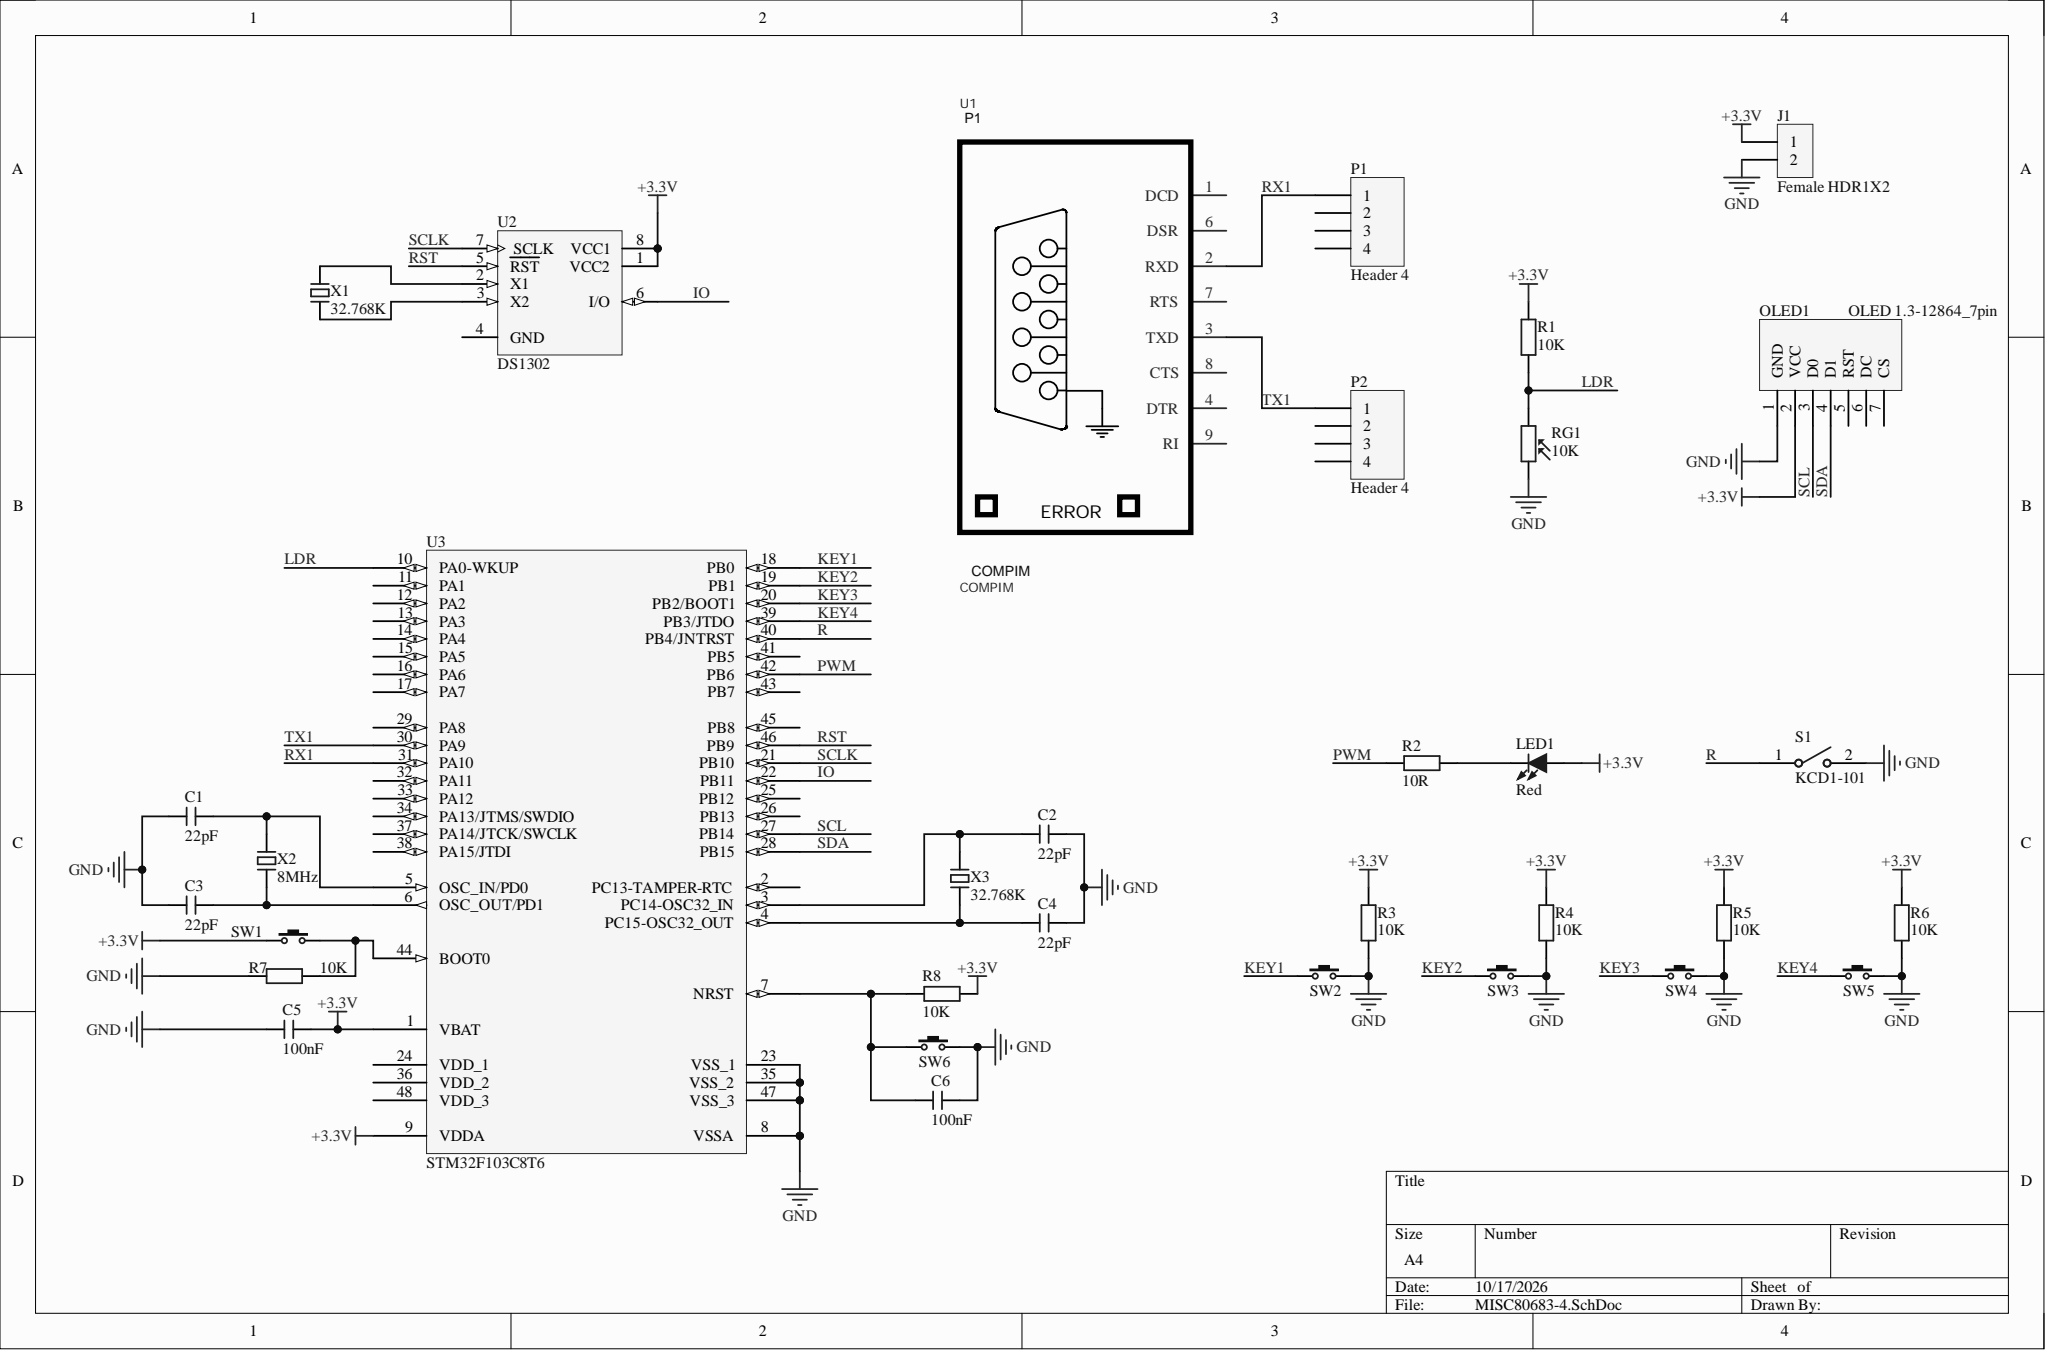Circuit board | Altium Designer | 33 parts | 25 nets
Bill of materials:
Comment,Description,Designator,Footprint,LibRef,Quantity
"22pF","Chip capacitor","C1, C2, C3, C4","C 0805_L","C","4"
"100nF","Chip capacitor","C5, C6","C 0805_L","C","2"
"Female HDR1X2","","J1","Fe-HDR1X2/2.54-S","Female HDR1X2","1"
"Red","Chip LED","LED1","LED 0805G","LED-SMD","1"
"OLED 1.3-12864_7pin","12864 dot-matrix display","OLED1","OLED 1.3-12864_7pin","OLED 1.3-12864_7pin","1"
"Header 4","Header, 4-Pin","P1, P2","Fe-HDR1X4/2.54-S","Header 4","2"
"10K","Chip resistor","R1, R3, R4, R5, R6, R7, R8","R 0805_L","R","7"
"10R","Chip resistor","R2","R 0805_L","R","1"
"10K","Photoresistor","RG1","RG5528","RG","1"
"KCD1-101","1-circuit SPST boat-type switch","S1","CSW DIP-1P","KCD1-101","1"
"3x6x5","3x6 tactile switch","SW1, SW2, SW3, SW4, SW5, SW6","TSW SMD-3*6*2.5","TSW 3x6","6"
"COMPIM","","U1","Fe-HDR1X9/2.54-S","COMPIM","1"
"DS1302","Trickle Charge Timekeeping Chip","U2","SOP8","DS1302","1"
"STM32F103C8T6","","U3","LQFP48 7X7","STM32F103C8T6","1"
"32.768K","2-pin passive crystal","X1, X3","OSC 3215-2P","XTAL-2P","2"
"8MHz","2-pin passive crystal","X2","OSC 6035-2P","XTAL-2P","1"
Netlist (Protel format):
[
C1
C 0805_L
22pF



]
[
C2
C 0805_L
22pF



]
[
C3
C 0805_L
22pF



]
[
C4
C 0805_L
22pF



]
[
C5
C 0805_L
100nF



]
[
C6
C 0805_L
100nF



]
[
J1
Fe-HDR1X2/2.54-S
Female HDR1X2



]
[
LED1
LED 0805G
Red



]
[
OLED1
OLED 1.3-12864_7pin
OLED 1.3-12864_7pin



]
[
P1
Fe-HDR1X4/2.54-S
Header 4



]
[
P2
Fe-HDR1X4/2.54-S
Header 4



]
[
R1
R 0805_L
10K



]
[
R2
R 0805_L
10R



]
[
R3
R 0805_L
10K



]
[
R4
R 0805_L
10K



]
[
R5
R 0805_L
10K



]
[
R6
R 0805_L
10K



]
[
R7
R 0805_L
10K



]
[
R8
R 0805_L
10K



]
[
RG1
RG5528
10K



]
[
S1
CSW DIP-1P
KCD1-101



]
[
SW1
TSW SMD-3*6*2.5
3x6x5



]
[
SW2
TSW SMD-3*6*2.5
3x6x5



]
[
SW3
TSW SMD-3*6*2.5
3x6x5



]
[
SW4
TSW SMD-3*6*2.5
3x6x5



]
[
SW5
TSW SMD-3*6*2.5
3x6x5



]
[
SW6
TSW SMD-3*6*2.5
3x6x5



]
[
U1
Fe-HDR1X9/2.54-S
COMPIM



]
[
U2
SOP8
DS1302



]
[
U3
LQFP48 7X7
STM32F103C8T6



]
[
X1
OSC 3215-2P
32.768K



]
[
X2
OSC 6035-2P
8MHz



]
[
X3
OSC 3215-2P
32.768K



]
(
TX1
P2-1
U1-3
U3-30
)
(
SDA
OLED1-4
U3-28
)
(
SCLK
U2-7
U3-21
)
(
SCL
OLED1-3
U3-27
)
(
RX1
P1-1
U1-2
U3-31
)
(
RST
U2-5
U3-46
)
(
R
S1-1
U3-40
)
(
PWM
R2-2
U3-42
)
(
NetU2_3
U2-3
X1-1
)
(
NetU2_2
U2-2
X1-2
)
(
NetR7_2
R7-2
SW1-2
U3-44
)
(
NetLED1_2
LED1-2
R2-1
)
(
NetC6_1
C6-1
R8-1
SW6-1
U3-7
)
(
NetC4_1
C4-1
U3-4
X3-1
)
(
NetC3_2
C3-2
U3-6
X2-1
)
(
NetC2_1
C2-1
U3-3
X3-2
)
(
NetC1_2
C1-2
U3-5
X2-2
)
(
LDR
R1-1
RG1-2
U3-10
)
(
KEY4
SW5-1
U3-39
)
(
KEY3
SW4-1
U3-20
)
(
KEY2
SW3-1
U3-19
)
(
KEY1
SW2-1
U3-18
)
(
IO
U2-6
U3-22
)
(
GND
C1-1
C2-2
C3-1
C4-2
C5-2
C6-2
J1-2
OLED1-1
R3-1
R4-1
R5-1
R6-1
R7-1
RG1-1
S1-2
SW2-2
SW3-2
SW4-2
SW5-2
SW6-2
U3-8
U3-23
U3-35
U3-47
)
(
+3.3V
C5-1
J1-1
LED1-1
OLED1-2
R1-2
R3-2
R4-2
R5-2
R6-2
R8-2
SW1-1
U2-1
U2-8
U3-1
U3-9
)